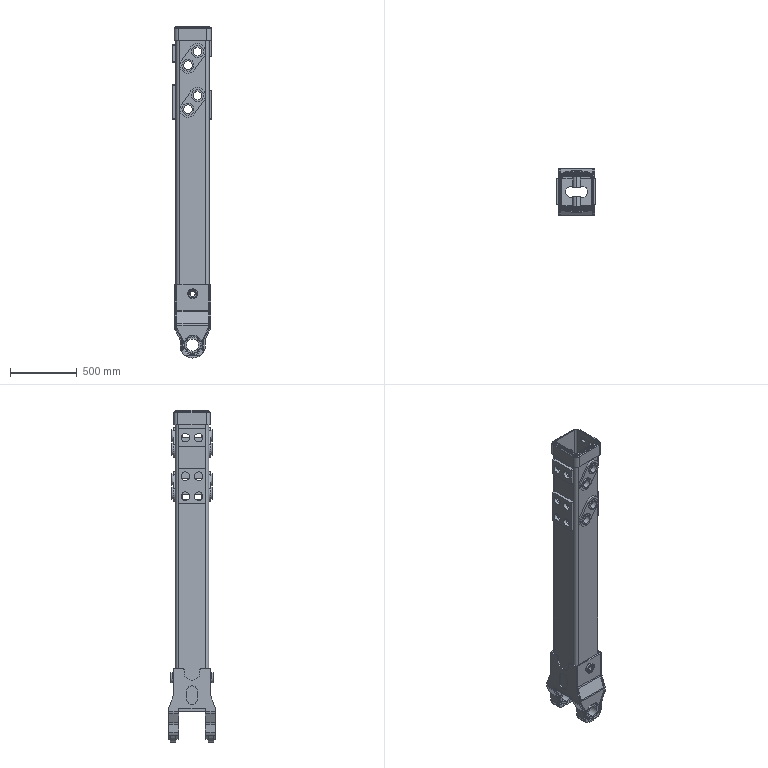Part | SolidWorks | features Cut 9, ReferencePattern 4, MirrorCompFeat 3, Chamfer 1, LocalLPattern 1, MirrorPattern 1, RefAxis 1 | 31 solids | 881 faces | box 291 x 352 x 2492 mm | volume 37081003 mm3 | plane 403 | cylinder 368 | cone 110 | commonest cylinder face diameters 80 x72 10 x64 60 x44 64 x44 10.2 x32 90 x20